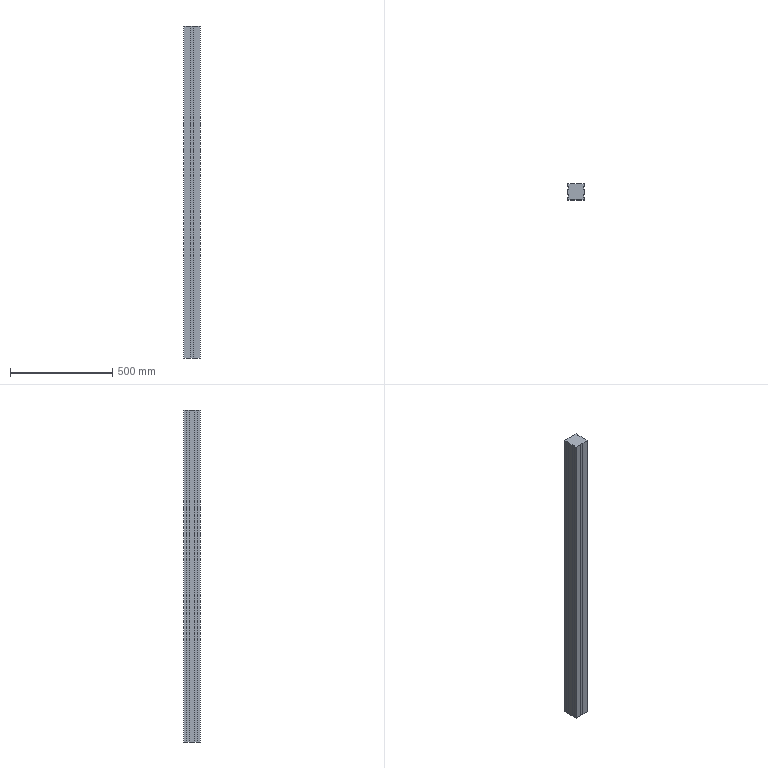Part | STEP file | xingcai80x80x1620 | 1 solid | 30 faces | box 80 x 80 x 1620 mm | volume 10095840 mm3 | plane 30